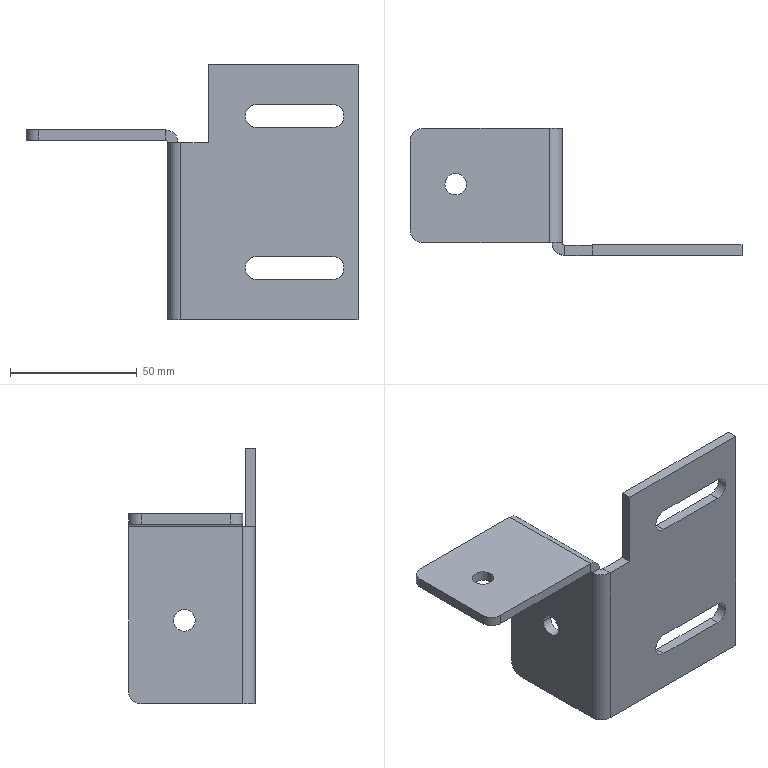Part | SolidWorks | features ICE 6, EdgeFlange 1, Fillet 1, FlatPattern 1, SMBaseFlange 1, SheetMetal 1 | 1 solid | 39 faces | box 131 x 50 x 101 mm | volume 48396 mm3 | plane 24 | cylinder 15 | commonest cylinder face diameters 10 x5 8.5 x4 9 x4 2 x2
STEP:
#1=CARTESIAN_POINT('',(-24.207,-4.491,33.));
#2=VERTEX_POINT('',#1);
#3=CARTESIAN_POINT('',(-24.207,4.009,33.));
#4=VERTEX_POINT('',#3);
#5=CARTESIAN_POINT('',(-24.207,-0.2414,33.));
#6=DIRECTION('',(1.,0.,0.));
#7=DIRECTION('',(0.,1.,0.));
#8=AXIS2_PLACEMENT_3D('',#5,#6,#7);
#9=CIRCLE('',#8,4.25);
#10=EDGE_CURVE('',#2,#4,#9,.T.);
#11=ORIENTED_EDGE('',*,*,#10,.F.);
#12=CARTESIAN_POINT('',(-20.207,-4.491,33.));
#13=VERTEX_POINT('',#12);
#14=CARTESIAN_POINT('',(-30.207,-4.491,33.));
#15=DIRECTION('',(1.,0.,0.));
#16=VECTOR('',#15,1000.);
#17=LINE('',#14,#16);
#18=EDGE_CURVE('',#2,#13,#17,.T.);
#19=ORIENTED_EDGE('',*,*,#18,.T.);
#20=CARTESIAN_POINT('',(-20.207,4.009,33.));
#21=VERTEX_POINT('',#20);
#22=CARTESIAN_POINT('',(-20.207,-0.2414,33.));
#23=DIRECTION('',(1.,0.,0.));
#24=DIRECTION('',(0.,1.,0.));
#25=AXIS2_PLACEMENT_3D('',#22,#23,#24);
#26=CIRCLE('',#25,4.25);
#27=EDGE_CURVE('',#13,#21,#26,.T.);
#28=ORIENTED_EDGE('',*,*,#27,.T.);
#29=CARTESIAN_POINT('',(-30.207,4.009,33.));
#30=DIRECTION('',(1.,0.,0.));
#31=VECTOR('',#30,1000.);
#32=LINE('',#29,#31);
#33=EDGE_CURVE('',#4,#21,#32,.T.);
#34=ORIENTED_EDGE('',*,*,#33,.F.);
#35=EDGE_LOOP('',(#11,#19,#28,#34));
#36=FACE_OUTER_BOUND('',#35,.T.);
#37=CARTESIAN_POINT('',(-30.207,-0.2414,33.));
#38=DIRECTION('',(1.,0.,0.));
#39=DIRECTION('',(0.,1.,0.));
#40=AXIS2_PLACEMENT_3D('',#37,#38,#39);
#41=CYLINDRICAL_SURFACE('',#40,4.25);
#42=ADVANCED_FACE('',(#36),#41,.F.);
#43=CARTESIAN_POINT('',(-66.457,-0.2414,71.));
#44=VERTEX_POINT('',#43);
#45=CARTESIAN_POINT('',(-57.957,-0.2414,71.));
#46=VERTEX_POINT('',#45);
#47=CARTESIAN_POINT('',(-62.207,-0.2414,71.));
#48=DIRECTION('',(0.,0.,1.));
#49=DIRECTION('',(1.,0.,0.));
#50=AXIS2_PLACEMENT_3D('',#47,#48,#49);
#51=CIRCLE('',#50,4.25);
#52=EDGE_CURVE('',#44,#46,#51,.T.);
#53=ORIENTED_EDGE('',*,*,#52,.F.);
#54=CARTESIAN_POINT('',(-66.457,-0.2414,75.));
#55=VERTEX_POINT('',#54);
#56=CARTESIAN_POINT('',(-66.457,-0.2414,65.));
#57=DIRECTION('',(0.,0.,1.));
#58=VECTOR('',#57,1000.);
#59=LINE('',#56,#58);
#60=EDGE_CURVE('',#44,#55,#59,.T.);
#61=ORIENTED_EDGE('',*,*,#60,.T.);
#62=CARTESIAN_POINT('',(-57.957,-0.2414,75.));
#63=VERTEX_POINT('',#62);
#64=CARTESIAN_POINT('',(-62.207,-0.2414,75.));
#65=DIRECTION('',(0.,0.,1.));
#66=DIRECTION('',(1.,0.,0.));
#67=AXIS2_PLACEMENT_3D('',#64,#65,#66);
#68=CIRCLE('',#67,4.25);
#69=EDGE_CURVE('',#55,#63,#68,.T.);
#70=ORIENTED_EDGE('',*,*,#69,.T.);
#71=CARTESIAN_POINT('',(-57.957,-0.2414,65.));
#72=DIRECTION('',(0.,0.,1.));
#73=VECTOR('',#72,1000.);
#74=LINE('',#71,#73);
#75=EDGE_CURVE('',#46,#63,#74,.T.);
#76=ORIENTED_EDGE('',*,*,#75,.F.);
#77=EDGE_LOOP('',(#53,#61,#70,#76));
#78=FACE_OUTER_BOUND('',#77,.T.);
#79=CARTESIAN_POINT('',(-62.207,-0.2414,65.));
#80=DIRECTION('',(0.,0.,1.));
#81=DIRECTION('',(1.,0.,0.));
#82=AXIS2_PLACEMENT_3D('',#79,#80,#81);
#83=CYLINDRICAL_SURFACE('',#82,4.25);
#84=ADVANCED_FACE('',(#78),#83,.F.);
#85=CARTESIAN_POINT('',(-8.207,-24.241,70.));
#86=VERTEX_POINT('',#85);
#87=CARTESIAN_POINT('',(-19.207,-24.241,70.));
#88=VERTEX_POINT('',#87);
#89=CARTESIAN_POINT('',(-24.207,-24.241,70.));
#90=DIRECTION('',(-1.,0.,0.));
#91=VECTOR('',#90,1000.);
#92=LINE('',#89,#91);
#93=EDGE_CURVE('',#86,#88,#92,.T.);
#94=ORIENTED_EDGE('',*,*,#93,.T.);
#95=CARTESIAN_POINT('',(-19.207,-28.241,70.));
#96=VERTEX_POINT('',#95);
#97=CARTESIAN_POINT('',(-19.207,-24.241,70.));
#98=DIRECTION('',(0.,-1.,0.));
#99=VECTOR('',#98,1000.);
#100=LINE('',#97,#99);
#101=EDGE_CURVE('',#88,#96,#100,.T.);
#102=ORIENTED_EDGE('',*,*,#101,.T.);
#103=CARTESIAN_POINT('',(-8.207,-28.241,70.));
#104=VERTEX_POINT('',#103);
#105=CARTESIAN_POINT('',(-8.207,-28.241,70.));
#106=DIRECTION('',(-1.,0.,0.));
#107=VECTOR('',#106,1000.);
#108=LINE('',#105,#107);
#109=EDGE_CURVE('',#104,#96,#108,.T.);
#110=ORIENTED_EDGE('',*,*,#109,.F.);
#111=CARTESIAN_POINT('',(-8.207,-28.241,70.));
#112=DIRECTION('',(0.,1.,0.));
#113=VECTOR('',#112,1000.);
#114=LINE('',#111,#113);
#115=EDGE_CURVE('',#104,#86,#114,.T.);
#116=ORIENTED_EDGE('',*,*,#115,.T.);
#117=EDGE_LOOP('',(#94,#102,#110,#116));
#118=FACE_OUTER_BOUND('',#117,.T.);
#119=CARTESIAN_POINT('',(-8.207,-28.241,70.));
#120=DIRECTION('',(0.,0.,-1.));
#121=DIRECTION('',(-1.,0.,0.));
#122=AXIS2_PLACEMENT_3D('',#119,#120,#121);
#123=PLANE('',#122);
#124=ADVANCED_FACE('',(#118),#123,.F.);
#125=CARTESIAN_POINT('',(-19.207,-28.241,0.));
#126=VERTEX_POINT('',#125);
#127=CARTESIAN_POINT('',(-19.207,-24.241,0.));
#128=VERTEX_POINT('',#127);
#129=CARTESIAN_POINT('',(-19.207,-28.241,0.));
#130=DIRECTION('',(0.,1.,0.));
#131=VECTOR('',#130,1000.);
#132=LINE('',#129,#131);
#133=EDGE_CURVE('',#126,#128,#132,.T.);
#134=ORIENTED_EDGE('',*,*,#133,.F.);
#135=CARTESIAN_POINT('',(-24.207,-23.241,0.));
#136=VERTEX_POINT('',#135);
#137=CARTESIAN_POINT('',(-19.207,-23.241,0.));
#138=DIRECTION('',(0.,0.,1.));
#139=DIRECTION('',(-1.,0.,0.));
#140=AXIS2_PLACEMENT_3D('',#137,#138,#139);
#141=CIRCLE('',#140,5.);
#142=EDGE_CURVE('',#136,#126,#141,.T.);
#143=ORIENTED_EDGE('',*,*,#142,.F.);
#144=CARTESIAN_POINT('',(-20.207,-23.241,0.));
#145=VERTEX_POINT('',#144);
#146=CARTESIAN_POINT('',(-20.207,-23.241,0.));
#147=DIRECTION('',(-1.,0.,0.));
#148=VECTOR('',#147,1000.);
#149=LINE('',#146,#148);
#150=EDGE_CURVE('',#145,#136,#149,.T.);
#151=ORIENTED_EDGE('',*,*,#150,.F.);
#152=CARTESIAN_POINT('',(-19.207,-23.241,0.));
#153=DIRECTION('',(0.,0.,1.));
#154=DIRECTION('',(1.,0.,0.));
#155=AXIS2_PLACEMENT_3D('',#152,#153,#154);
#156=CIRCLE('',#155,1.);
#157=EDGE_CURVE('',#145,#128,#156,.T.);
#158=ORIENTED_EDGE('',*,*,#157,.T.);
#159=EDGE_LOOP('',(#134,#143,#151,#158));
#160=FACE_OUTER_BOUND('',#159,.T.);
#161=CARTESIAN_POINT('',(-19.207,-28.241,0.));
#162=DIRECTION('',(0.,0.,-1.));
#163=DIRECTION('',(-1.,0.,0.));
#164=AXIS2_PLACEMENT_3D('',#161,#162,#163);
#165=PLANE('',#164);
#166=ADVANCED_FACE('',(#160),#165,.T.);
#167=CARTESIAN_POINT('',(50.793,-28.241,0.));
#168=VERTEX_POINT('',#167);
#169=CARTESIAN_POINT('',(50.793,-24.241,0.));
#170=VERTEX_POINT('',#169);
#171=CARTESIAN_POINT('',(50.793,-34.241,0.));
#172=DIRECTION('',(0.,1.,0.));
#173=VECTOR('',#172,1000.);
#174=LINE('',#171,#173);
#175=EDGE_CURVE('',#168,#170,#174,.T.);
#176=ORIENTED_EDGE('',*,*,#175,.F.);
#177=CARTESIAN_POINT('',(-24.207,-28.241,0.));
#178=DIRECTION('',(1.,0.,0.));
#179=VECTOR('',#178,1000.);
#180=LINE('',#177,#179);
#181=EDGE_CURVE('',#126,#168,#180,.T.);
#182=ORIENTED_EDGE('',*,*,#181,.F.);
#183=ORIENTED_EDGE('',*,*,#133,.T.);
#184=CARTESIAN_POINT('',(-24.207,-24.241,0.));
#185=DIRECTION('',(1.,0.,0.));
#186=VECTOR('',#185,1000.);
#187=LINE('',#184,#186);
#188=EDGE_CURVE('',#128,#170,#187,.T.);
#189=ORIENTED_EDGE('',*,*,#188,.T.);
#190=EDGE_LOOP('',(#176,#182,#183,#189));
#191=FACE_OUTER_BOUND('',#190,.T.);
#192=CARTESIAN_POINT('',(-20.207,-23.241,0.));
#193=DIRECTION('',(0.,0.,-1.));
#194=DIRECTION('',(-1.,0.,0.));
#195=AXIS2_PLACEMENT_3D('',#192,#193,#194);
#196=PLANE('',#195);
#197=ADVANCED_FACE('',(#191),#196,.T.);
#198=CARTESIAN_POINT('',(40.793,-28.241,16.));
#199=VERTEX_POINT('',#198);
#200=CARTESIAN_POINT('',(10.793,-28.241,16.));
#201=VERTEX_POINT('',#200);
#202=CARTESIAN_POINT('',(-24.207,-28.241,16.));
#203=DIRECTION('',(-1.,0.,0.));
#204=VECTOR('',#203,1000.);
#205=LINE('',#202,#204);
#206=EDGE_CURVE('',#199,#201,#205,.T.);
#207=ORIENTED_EDGE('',*,*,#206,.T.);
#208=CARTESIAN_POINT('',(10.793,-28.241,25.));
#209=VERTEX_POINT('',#208);
#210=CARTESIAN_POINT('',(10.793,-28.241,20.5));
#211=DIRECTION('',(0.,1.,0.));
#212=DIRECTION('',(0.,0.,1.));
#213=AXIS2_PLACEMENT_3D('',#210,#211,#212);
#214=CIRCLE('',#213,4.5);
#215=EDGE_CURVE('',#201,#209,#214,.T.);
#216=ORIENTED_EDGE('',*,*,#215,.T.);
#217=CARTESIAN_POINT('',(40.793,-28.241,25.));
#218=VERTEX_POINT('',#217);
#219=CARTESIAN_POINT('',(-24.207,-28.241,25.));
#220=DIRECTION('',(1.,0.,0.));
#221=VECTOR('',#220,1000.);
#222=LINE('',#219,#221);
#223=EDGE_CURVE('',#209,#218,#222,.T.);
#224=ORIENTED_EDGE('',*,*,#223,.T.);
#225=CARTESIAN_POINT('',(40.793,-28.241,20.5));
#226=DIRECTION('',(0.,1.,0.));
#227=DIRECTION('',(0.,0.,1.));
#228=AXIS2_PLACEMENT_3D('',#225,#226,#227);
#229=CIRCLE('',#228,4.5);
#230=EDGE_CURVE('',#218,#199,#229,.T.);
#231=ORIENTED_EDGE('',*,*,#230,.T.);
#232=EDGE_LOOP('',(#207,#216,#224,#231));
#233=FACE_BOUND('',#232,.T.);
#234=CARTESIAN_POINT('',(40.793,-28.241,76.));
#235=VERTEX_POINT('',#234);
#236=CARTESIAN_POINT('',(10.793,-28.241,76.));
#237=VERTEX_POINT('',#236);
#238=CARTESIAN_POINT('',(-24.207,-28.241,76.));
#239=DIRECTION('',(-1.,0.,0.));
#240=VECTOR('',#239,1000.);
#241=LINE('',#238,#240);
#242=EDGE_CURVE('',#235,#237,#241,.T.);
#243=ORIENTED_EDGE('',*,*,#242,.T.);
#244=CARTESIAN_POINT('',(10.793,-28.241,85.));
#245=VERTEX_POINT('',#244);
#246=CARTESIAN_POINT('',(10.793,-28.241,80.5));
#247=DIRECTION('',(0.,1.,0.));
#248=DIRECTION('',(0.,0.,1.));
#249=AXIS2_PLACEMENT_3D('',#246,#247,#248);
#250=CIRCLE('',#249,4.5);
#251=EDGE_CURVE('',#237,#245,#250,.T.);
#252=ORIENTED_EDGE('',*,*,#251,.T.);
#253=CARTESIAN_POINT('',(40.793,-28.241,85.));
#254=VERTEX_POINT('',#253);
#255=CARTESIAN_POINT('',(-24.207,-28.241,85.));
#256=DIRECTION('',(1.,0.,0.));
#257=VECTOR('',#256,1000.);
#258=LINE('',#255,#257);
#259=EDGE_CURVE('',#245,#254,#258,.T.);
#260=ORIENTED_EDGE('',*,*,#259,.T.);
#261=CARTESIAN_POINT('',(40.793,-28.241,80.5));
#262=DIRECTION('',(0.,1.,0.));
#263=DIRECTION('',(0.,0.,1.));
#264=AXIS2_PLACEMENT_3D('',#261,#262,#263);
#265=CIRCLE('',#264,4.5);
#266=EDGE_CURVE('',#254,#235,#265,.T.);
#267=ORIENTED_EDGE('',*,*,#266,.T.);
#268=EDGE_LOOP('',(#243,#252,#260,#267));
#269=FACE_BOUND('',#268,.T.);
#270=ORIENTED_EDGE('',*,*,#181,.T.);
#271=CARTESIAN_POINT('',(50.793,-28.241,101.));
#272=VERTEX_POINT('',#271);
#273=CARTESIAN_POINT('',(50.793,-28.241,125.));
#274=DIRECTION('',(0.,0.,1.));
#275=VECTOR('',#274,1000.);
#276=LINE('',#273,#275);
#277=EDGE_CURVE('',#168,#272,#276,.T.);
#278=ORIENTED_EDGE('',*,*,#277,.T.);
#279=CARTESIAN_POINT('',(-8.207,-28.241,101.));
#280=VERTEX_POINT('',#279);
#281=CARTESIAN_POINT('',(-24.207,-28.241,101.));
#282=DIRECTION('',(-1.,0.,0.));
#283=VECTOR('',#282,1000.);
#284=LINE('',#281,#283);
#285=EDGE_CURVE('',#272,#280,#284,.T.);
#286=ORIENTED_EDGE('',*,*,#285,.T.);
#287=CARTESIAN_POINT('',(-8.207,-28.241,125.));
#288=DIRECTION('',(0.,0.,-1.));
#289=VECTOR('',#288,1000.);
#290=LINE('',#287,#289);
#291=EDGE_CURVE('',#280,#104,#290,.T.);
#292=ORIENTED_EDGE('',*,*,#291,.T.);
#293=ORIENTED_EDGE('',*,*,#109,.T.);
#294=CARTESIAN_POINT('',(-19.207,-28.241,125.));
#295=DIRECTION('',(0.,0.,-1.));
#296=VECTOR('',#295,1000.);
#297=LINE('',#294,#296);
#298=EDGE_CURVE('',#96,#126,#297,.T.);
#299=ORIENTED_EDGE('',*,*,#298,.T.);
#300=EDGE_LOOP('',(#270,#278,#286,#292,#293,#299));
#301=FACE_OUTER_BOUND('',#300,.T.);
#302=CARTESIAN_POINT('',(-24.207,-28.241,125.));
#303=DIRECTION('',(0.,1.,0.));
#304=DIRECTION('',(0.,0.,1.));
#305=AXIS2_PLACEMENT_3D('',#302,#303,#304);
#306=PLANE('',#305);
#307=ADVANCED_FACE('',(#233,#269,#301),#306,.F.);
#308=CARTESIAN_POINT('',(10.793,-24.241,16.));
#309=VERTEX_POINT('',#308);
#310=CARTESIAN_POINT('',(10.793,-24.241,25.));
#311=VERTEX_POINT('',#310);
#312=CARTESIAN_POINT('',(10.793,-24.241,20.5));
#313=DIRECTION('',(0.,1.,0.));
#314=DIRECTION('',(0.,0.,1.));
#315=AXIS2_PLACEMENT_3D('',#312,#313,#314);
#316=CIRCLE('',#315,4.5);
#317=EDGE_CURVE('',#309,#311,#316,.T.);
#318=ORIENTED_EDGE('',*,*,#317,.F.);
#319=CARTESIAN_POINT('',(40.793,-24.241,16.));
#320=VERTEX_POINT('',#319);
#321=CARTESIAN_POINT('',(10.793,-24.241,16.));
#322=DIRECTION('',(-1.,0.,0.));
#323=VECTOR('',#322,1000.);
#324=LINE('',#321,#323);
#325=EDGE_CURVE('',#320,#309,#324,.T.);
#326=ORIENTED_EDGE('',*,*,#325,.F.);
#327=CARTESIAN_POINT('',(40.793,-24.241,25.));
#328=VERTEX_POINT('',#327);
#329=CARTESIAN_POINT('',(40.793,-24.241,20.5));
#330=DIRECTION('',(0.,1.,0.));
#331=DIRECTION('',(0.,0.,1.));
#332=AXIS2_PLACEMENT_3D('',#329,#330,#331);
#333=CIRCLE('',#332,4.5);
#334=EDGE_CURVE('',#328,#320,#333,.T.);
#335=ORIENTED_EDGE('',*,*,#334,.F.);
#336=CARTESIAN_POINT('',(10.793,-24.241,25.));
#337=DIRECTION('',(1.,0.,0.));
#338=VECTOR('',#337,1000.);
#339=LINE('',#336,#338);
#340=EDGE_CURVE('',#311,#328,#339,.T.);
#341=ORIENTED_EDGE('',*,*,#340,.F.);
#342=EDGE_LOOP('',(#318,#326,#335,#341));
#343=FACE_BOUND('',#342,.T.);
#344=CARTESIAN_POINT('',(10.793,-24.241,76.));
#345=VERTEX_POINT('',#344);
#346=CARTESIAN_POINT('',(10.793,-24.241,85.));
#347=VERTEX_POINT('',#346);
#348=CARTESIAN_POINT('',(10.793,-24.241,80.5));
#349=DIRECTION('',(0.,1.,0.));
#350=DIRECTION('',(0.,0.,-1.));
#351=AXIS2_PLACEMENT_3D('',#348,#349,#350);
#352=CIRCLE('',#351,4.5);
#353=EDGE_CURVE('',#345,#347,#352,.T.);
#354=ORIENTED_EDGE('',*,*,#353,.F.);
#355=CARTESIAN_POINT('',(40.793,-24.241,76.));
#356=VERTEX_POINT('',#355);
#357=CARTESIAN_POINT('',(10.793,-24.241,76.));
#358=DIRECTION('',(-1.,0.,0.));
#359=VECTOR('',#358,1000.);
#360=LINE('',#357,#359);
#361=EDGE_CURVE('',#356,#345,#360,.T.);
#362=ORIENTED_EDGE('',*,*,#361,.F.);
#363=CARTESIAN_POINT('',(40.793,-24.241,85.));
#364=VERTEX_POINT('',#363);
#365=CARTESIAN_POINT('',(40.793,-24.241,80.5));
#366=DIRECTION('',(0.,1.,0.));
#367=DIRECTION('',(0.,0.,-1.));
#368=AXIS2_PLACEMENT_3D('',#365,#366,#367);
#369=CIRCLE('',#368,4.5);
#370=EDGE_CURVE('',#364,#356,#369,.T.);
#371=ORIENTED_EDGE('',*,*,#370,.F.);
#372=CARTESIAN_POINT('',(10.793,-24.241,85.));
#373=DIRECTION('',(1.,0.,0.));
#374=VECTOR('',#373,1000.);
#375=LINE('',#372,#374);
#376=EDGE_CURVE('',#347,#364,#375,.T.);
#377=ORIENTED_EDGE('',*,*,#376,.F.);
#378=EDGE_LOOP('',(#354,#362,#371,#377));
#379=FACE_BOUND('',#378,.T.);
#380=CARTESIAN_POINT('',(50.793,-24.241,101.));
#381=VERTEX_POINT('',#380);
#382=CARTESIAN_POINT('',(50.793,-24.241,0.));
#383=DIRECTION('',(0.,0.,1.));
#384=VECTOR('',#383,1000.);
#385=LINE('',#382,#384);
#386=EDGE_CURVE('',#170,#381,#385,.T.);
#387=ORIENTED_EDGE('',*,*,#386,.F.);
#388=ORIENTED_EDGE('',*,*,#188,.F.);
#389=CARTESIAN_POINT('',(-19.207,-24.241,125.));
#390=DIRECTION('',(0.,0.,-1.));
#391=VECTOR('',#390,1000.);
#392=LINE('',#389,#391);
#393=EDGE_CURVE('',#88,#128,#392,.T.);
#394=ORIENTED_EDGE('',*,*,#393,.F.);
#395=ORIENTED_EDGE('',*,*,#93,.F.);
#396=CARTESIAN_POINT('',(-8.207,-24.241,101.));
#397=VERTEX_POINT('',#396);
#398=CARTESIAN_POINT('',(-8.207,-24.241,125.));
#399=DIRECTION('',(0.,0.,-1.));
#400=VECTOR('',#399,1000.);
#401=LINE('',#398,#400);
#402=EDGE_CURVE('',#397,#86,#401,.T.);
#403=ORIENTED_EDGE('',*,*,#402,.F.);
#404=CARTESIAN_POINT('',(-8.207,-24.241,101.));
#405=DIRECTION('',(-1.,0.,0.));
#406=VECTOR('',#405,1000.);
#407=LINE('',#404,#406);
#408=EDGE_CURVE('',#381,#397,#407,.T.);
#409=ORIENTED_EDGE('',*,*,#408,.F.);
#410=EDGE_LOOP('',(#387,#388,#394,#395,#403,#409));
#411=FACE_OUTER_BOUND('',#410,.T.);
#412=CARTESIAN_POINT('',(-24.207,-24.241,125.));
#413=DIRECTION('',(0.,1.,0.));
#414=DIRECTION('',(0.,0.,1.));
#415=AXIS2_PLACEMENT_3D('',#412,#413,#414);
#416=PLANE('',#415);
#417=ADVANCED_FACE('',(#343,#379,#411),#416,.T.);
#418=CARTESIAN_POINT('',(-20.207,-23.241,70.));
#419=VERTEX_POINT('',#418);
#420=CARTESIAN_POINT('',(-19.207,-23.241,70.));
#421=DIRECTION('',(0.,0.,-1.));
#422=DIRECTION('',(-1.,0.,0.));
#423=AXIS2_PLACEMENT_3D('',#420,#421,#422);
#424=CIRCLE('',#423,1.);
#425=EDGE_CURVE('',#88,#419,#424,.T.);
#426=ORIENTED_EDGE('',*,*,#425,.F.);
#427=ORIENTED_EDGE('',*,*,#393,.T.);
#428=ORIENTED_EDGE('',*,*,#157,.F.);
#429=CARTESIAN_POINT('',(-20.207,-23.241,125.));
#430=DIRECTION('',(0.,0.,-1.));
#431=VECTOR('',#430,1000.);
#432=LINE('',#429,#431);
#433=EDGE_CURVE('',#419,#145,#432,.T.);
#434=ORIENTED_EDGE('',*,*,#433,.F.);
#435=EDGE_LOOP('',(#426,#427,#428,#434));
#436=FACE_OUTER_BOUND('',#435,.T.);
#437=CARTESIAN_POINT('',(-19.207,-23.241,125.));
#438=DIRECTION('',(0.,0.,-1.));
#439=DIRECTION('',(-1.,0.,0.));
#440=AXIS2_PLACEMENT_3D('',#437,#438,#439);
#441=CYLINDRICAL_SURFACE('',#440,1.);
#442=ADVANCED_FACE('',(#436),#441,.F.);
#443=CARTESIAN_POINT('',(-20.207,-0.2414,33.));
#444=DIRECTION('',(1.,0.,0.));
#445=DIRECTION('',(0.,1.,0.));
#446=AXIS2_PLACEMENT_3D('',#443,#444,#445);
#447=CIRCLE('',#446,4.25);
#448=EDGE_CURVE('',#21,#13,#447,.T.);
#449=ORIENTED_EDGE('',*,*,#448,.F.);
#450=ORIENTED_EDGE('',*,*,#27,.F.);
#451=EDGE_LOOP('',(#449,#450));
#452=FACE_BOUND('',#451,.T.);
#453=CARTESIAN_POINT('',(-20.207,16.759,0.));
#454=VERTEX_POINT('',#453);
#455=CARTESIAN_POINT('',(-20.207,21.759,0.));
#456=DIRECTION('',(0.,-1.,0.));
#457=VECTOR('',#456,1000.);
#458=LINE('',#455,#457);
#459=EDGE_CURVE('',#454,#145,#458,.T.);
#460=ORIENTED_EDGE('',*,*,#459,.F.);
#461=CARTESIAN_POINT('',(-20.207,21.759,5.));
#462=VERTEX_POINT('',#461);
#463=CARTESIAN_POINT('',(-20.207,16.759,5.));
#464=DIRECTION('',(1.,0.,0.));
#465=DIRECTION('',(0.,1.,0.));
#466=AXIS2_PLACEMENT_3D('',#463,#464,#465);
#467=CIRCLE('',#466,5.);
#468=EDGE_CURVE('',#454,#462,#467,.T.);
#469=ORIENTED_EDGE('',*,*,#468,.T.);
#470=CARTESIAN_POINT('',(-20.207,21.759,70.));
#471=VERTEX_POINT('',#470);
#472=CARTESIAN_POINT('',(-20.207,21.759,125.));
#473=DIRECTION('',(0.,0.,-1.));
#474=VECTOR('',#473,1000.);
#475=LINE('',#472,#474);
#476=EDGE_CURVE('',#471,#462,#475,.T.);
#477=ORIENTED_EDGE('',*,*,#476,.F.);
#478=CARTESIAN_POINT('',(-20.207,21.759,70.));
#479=DIRECTION('',(0.,1.,0.));
#480=VECTOR('',#479,1000.);
#481=LINE('',#478,#480);
#482=EDGE_CURVE('',#419,#471,#481,.T.);
#483=ORIENTED_EDGE('',*,*,#482,.F.);
#484=ORIENTED_EDGE('',*,*,#433,.T.);
#485=EDGE_LOOP('',(#460,#469,#477,#483,#484));
#486=FACE_OUTER_BOUND('',#485,.T.);
#487=CARTESIAN_POINT('',(-20.207,21.759,125.));
#488=DIRECTION('',(1.,0.,0.));
#489=DIRECTION('',(0.,1.,0.));
#490=AXIS2_PLACEMENT_3D('',#487,#488,#489);
#491=PLANE('',#490);
#492=ADVANCED_FACE('',(#452,#486),#491,.T.);
#493=ORIENTED_EDGE('',*,*,#476,.T.);
#494=CARTESIAN_POINT('',(-24.207,21.759,5.));
#495=VERTEX_POINT('',#494);
#496=CARTESIAN_POINT('',(-24.207,21.759,5.));
#497=DIRECTION('',(-1.,0.,0.));
#498=VECTOR('',#497,1000.);
#499=LINE('',#496,#498);
#500=EDGE_CURVE('',#462,#495,#499,.T.);
#501=ORIENTED_EDGE('',*,*,#500,.T.);
#502=CARTESIAN_POINT('',(-24.207,21.759,70.));
#503=VERTEX_POINT('',#502);
#504=CARTESIAN_POINT('',(-24.207,21.759,125.));
#505=DIRECTION('',(0.,0.,-1.));
#506=VECTOR('',#505,1000.);
#507=LINE('',#504,#506);
#508=EDGE_CURVE('',#503,#495,#507,.T.);
#509=ORIENTED_EDGE('',*,*,#508,.F.);
#510=CARTESIAN_POINT('',(-8.207,21.759,70.));
#511=DIRECTION('',(-1.,0.,0.));
#512=VECTOR('',#511,1000.);
#513=LINE('',#510,#512);
#514=EDGE_CURVE('',#471,#503,#513,.T.);
#515=ORIENTED_EDGE('',*,*,#514,.F.);
#516=EDGE_LOOP('',(#493,#501,#509,#515));
#517=FACE_OUTER_BOUND('',#516,.T.);
#518=CARTESIAN_POINT('',(-24.207,21.759,125.));
#519=DIRECTION('',(0.,1.,0.));
#520=DIRECTION('',(0.,0.,1.));
#521=AXIS2_PLACEMENT_3D('',#518,#519,#520);
#522=PLANE('',#521);
#523=ADVANCED_FACE('',(#517),#522,.T.);
#524=CARTESIAN_POINT('',(-24.207,-0.2414,33.));
#525=DIRECTION('',(1.,0.,0.));
#526=DIRECTION('',(0.,1.,0.));
#527=AXIS2_PLACEMENT_3D('',#524,#525,#526);
#528=CIRCLE('',#527,4.25);
#529=EDGE_CURVE('',#4,#2,#528,.T.);
#530=ORIENTED_EDGE('',*,*,#529,.T.);
#531=ORIENTED_EDGE('',*,*,#10,.T.);
#532=EDGE_LOOP('',(#530,#531));
#533=FACE_BOUND('',#532,.T.);
#534=ORIENTED_EDGE('',*,*,#508,.T.);
#535=CARTESIAN_POINT('',(-24.207,16.759,0.));
#536=VERTEX_POINT('',#535);
#537=CARTESIAN_POINT('',(-24.207,16.759,5.));
#538=DIRECTION('',(-1.,0.,0.));
#539=DIRECTION('',(0.,1.,0.));
#540=AXIS2_PLACEMENT_3D('',#537,#538,#539);
#541=CIRCLE('',#540,5.);
#542=EDGE_CURVE('',#495,#536,#541,.T.);
#543=ORIENTED_EDGE('',*,*,#542,.T.);
#544=CARTESIAN_POINT('',(-24.207,21.759,0.));
#545=DIRECTION('',(0.,-1.,0.));
#546=VECTOR('',#545,1000.);
#547=LINE('',#544,#546);
#548=EDGE_CURVE('',#536,#136,#547,.T.);
#549=ORIENTED_EDGE('',*,*,#548,.T.);
#550=CARTESIAN_POINT('',(-24.207,-23.241,70.));
#551=VERTEX_POINT('',#550);
#552=CARTESIAN_POINT('',(-24.207,-23.241,125.));
#553=DIRECTION('',(0.,0.,-1.));
#554=VECTOR('',#553,1000.);
#555=LINE('',#552,#554);
#556=EDGE_CURVE('',#551,#136,#555,.T.);
#557=ORIENTED_EDGE('',*,*,#556,.F.);
#558=CARTESIAN_POINT('',(-24.207,21.759,70.));
#559=DIRECTION('',(0.,1.,0.));
#560=VECTOR('',#559,1000.);
#561=LINE('',#558,#560);
#562=EDGE_CURVE('',#551,#503,#561,.T.);
#563=ORIENTED_EDGE('',*,*,#562,.T.);
#564=EDGE_LOOP('',(#534,#543,#549,#557,#563));
#565=FACE_OUTER_BOUND('',#564,.T.);
#566=CARTESIAN_POINT('',(-24.207,21.759,125.));
#567=DIRECTION('',(1.,0.,0.));
#568=DIRECTION('',(0.,1.,0.));
#569=AXIS2_PLACEMENT_3D('',#566,#567,#568);
#570=PLANE('',#569);
#571=ADVANCED_FACE('',(#533,#565),#570,.F.);
#572=ORIENTED_EDGE('',*,*,#298,.F.);
#573=CARTESIAN_POINT('',(-19.207,-23.241,70.));
#574=DIRECTION('',(0.,0.,-1.));
#575=DIRECTION('',(-1.,0.,0.));
#576=AXIS2_PLACEMENT_3D('',#573,#574,#575);
#577=CIRCLE('',#576,5.);
#578=EDGE_CURVE('',#96,#551,#577,.T.);
#579=ORIENTED_EDGE('',*,*,#578,.T.);
#580=ORIENTED_EDGE('',*,*,#556,.T.);
#581=ORIENTED_EDGE('',*,*,#142,.T.);
#582=EDGE_LOOP('',(#572,#579,#580,#581));
#583=FACE_OUTER_BOUND('',#582,.T.);
#584=CARTESIAN_POINT('',(-19.207,-23.241,125.));
#585=DIRECTION('',(0.,0.,-1.));
#586=DIRECTION('',(-1.,0.,0.));
#587=AXIS2_PLACEMENT_3D('',#584,#585,#586);
#588=CYLINDRICAL_SURFACE('',#587,5.);
#589=ADVANCED_FACE('',(#583),#588,.T.);
#590=ORIENTED_EDGE('',*,*,#548,.F.);
#591=CARTESIAN_POINT('',(-20.207,16.759,0.));
#592=DIRECTION('',(1.,0.,0.));
#593=VECTOR('',#592,1000.);
#594=LINE('',#591,#593);
#595=EDGE_CURVE('',#536,#454,#594,.T.);
#596=ORIENTED_EDGE('',*,*,#595,.T.);
#597=ORIENTED_EDGE('',*,*,#459,.T.);
#598=ORIENTED_EDGE('',*,*,#150,.T.);
#599=EDGE_LOOP('',(#590,#596,#597,#598));
#600=FACE_OUTER_BOUND('',#599,.T.);
#601=CARTESIAN_POINT('',(-19.207,-23.241,0.));
#602=DIRECTION('',(0.,0.,1.));
#603=DIRECTION('',(1.,0.,0.));
#604=AXIS2_PLACEMENT_3D('',#601,#602,#603);
#605=PLANE('',#604);
#606=ADVANCED_FACE('',(#600),#605,.F.);
#607=CARTESIAN_POINT('',(-24.207,-23.241,70.));
#608=DIRECTION('',(1.,0.,0.));
#609=VECTOR('',#608,1000.);
#610=LINE('',#607,#609);
#611=EDGE_CURVE('',#551,#419,#610,.T.);
#612=ORIENTED_EDGE('',*,*,#611,.F.);
#613=ORIENTED_EDGE('',*,*,#578,.F.);
#614=ORIENTED_EDGE('',*,*,#101,.F.);
#615=ORIENTED_EDGE('',*,*,#425,.T.);
#616=EDGE_LOOP('',(#612,#613,#614,#615));
#617=FACE_OUTER_BOUND('',#616,.T.);
#618=CARTESIAN_POINT('',(-8.207,-28.241,70.));
#619=DIRECTION('',(0.,0.,-1.));
#620=DIRECTION('',(-1.,0.,0.));
#621=AXIS2_PLACEMENT_3D('',#618,#619,#620);
#622=PLANE('',#621);
#623=ADVANCED_FACE('',(#617),#622,.F.);
#624=ORIENTED_EDGE('',*,*,#291,.F.);
#625=CARTESIAN_POINT('',(-8.207,-28.241,101.));
#626=DIRECTION('',(0.,1.,0.));
#627=VECTOR('',#626,1000.);
#628=LINE('',#625,#627);
#629=EDGE_CURVE('',#280,#397,#628,.T.);
#630=ORIENTED_EDGE('',*,*,#629,.T.);
#631=ORIENTED_EDGE('',*,*,#402,.T.);
#632=ORIENTED_EDGE('',*,*,#115,.F.);
#633=EDGE_LOOP('',(#624,#630,#631,#632));
#634=FACE_OUTER_BOUND('',#633,.T.);
#635=CARTESIAN_POINT('',(-8.207,-28.241,125.));
#636=DIRECTION('',(1.,0.,0.));
#637=DIRECTION('',(0.,0.,-1.));
#638=AXIS2_PLACEMENT_3D('',#635,#636,#637);
#639=PLANE('',#638);
#640=ADVANCED_FACE('',(#634),#639,.F.);
#641=CARTESIAN_POINT('',(-25.207,-23.241,71.));
#642=VERTEX_POINT('',#641);
#643=CARTESIAN_POINT('',(-25.207,-23.241,75.));
#644=VERTEX_POINT('',#643);
#645=CARTESIAN_POINT('',(-25.207,-23.241,75.));
#646=DIRECTION('',(0.,0.,1.));
#647=VECTOR('',#646,1000.);
#648=LINE('',#645,#647);
#649=EDGE_CURVE('',#642,#644,#648,.T.);
#650=ORIENTED_EDGE('',*,*,#649,.F.);
#651=CARTESIAN_POINT('',(-25.207,-23.241,70.));
#652=DIRECTION('',(0.,-1.,0.));
#653=DIRECTION('',(0.,0.,1.));
#654=AXIS2_PLACEMENT_3D('',#651,#652,#653);
#655=CIRCLE('',#654,1.);
#656=EDGE_CURVE('',#551,#642,#655,.T.);
#657=ORIENTED_EDGE('',*,*,#656,.F.);
#658=ORIENTED_EDGE('',*,*,#611,.T.);
#659=CARTESIAN_POINT('',(-25.207,-23.241,70.));
#660=DIRECTION('',(0.,-1.,0.));
#661=DIRECTION('',(0.,0.,1.));
#662=AXIS2_PLACEMENT_3D('',#659,#660,#661);
#663=CIRCLE('',#662,5.);
#664=EDGE_CURVE('',#419,#644,#663,.T.);
#665=ORIENTED_EDGE('',*,*,#664,.T.);
#666=EDGE_LOOP('',(#650,#657,#658,#665));
#667=FACE_OUTER_BOUND('',#666,.T.);
#668=CARTESIAN_POINT('',(-25.207,-23.241,70.));
#669=DIRECTION('',(0.,-1.,0.));
#670=DIRECTION('',(0.,0.,-1.));
#671=AXIS2_PLACEMENT_3D('',#668,#669,#670);
#672=PLANE('',#671);
#673=ADVANCED_FACE('',(#667),#672,.T.);
#674=CARTESIAN_POINT('',(-25.207,21.759,71.));
#675=VERTEX_POINT('',#674);
#676=CARTESIAN_POINT('',(-25.207,21.759,70.));
#677=DIRECTION('',(0.,1.,0.));
#678=DIRECTION('',(0.,0.,1.));
#679=AXIS2_PLACEMENT_3D('',#676,#677,#678);
#680=CIRCLE('',#679,1.);
#681=EDGE_CURVE('',#675,#503,#680,.T.);
#682=ORIENTED_EDGE('',*,*,#681,.F.);
#683=CARTESIAN_POINT('',(-25.207,21.759,75.));
#684=VERTEX_POINT('',#683);
#685=CARTESIAN_POINT('',(-25.207,21.759,71.));
#686=DIRECTION('',(0.,0.,1.));
#687=VECTOR('',#686,1000.);
#688=LINE('',#685,#687);
#689=EDGE_CURVE('',#675,#684,#688,.T.);
#690=ORIENTED_EDGE('',*,*,#689,.T.);
#691=CARTESIAN_POINT('',(-25.207,21.759,70.));
#692=DIRECTION('',(0.,1.,0.));
#693=DIRECTION('',(0.,0.,1.));
#694=AXIS2_PLACEMENT_3D('',#691,#692,#693);
#695=CIRCLE('',#694,5.);
#696=EDGE_CURVE('',#684,#471,#695,.T.);
#697=ORIENTED_EDGE('',*,*,#696,.T.);
#698=ORIENTED_EDGE('',*,*,#514,.T.);
#699=EDGE_LOOP('',(#682,#690,#697,#698));
#700=FACE_OUTER_BOUND('',#699,.T.);
#701=CARTESIAN_POINT('',(-25.207,21.759,70.));
#702=DIRECTION('',(0.,-1.,0.));
#703=DIRECTION('',(0.,0.,-1.));
#704=AXIS2_PLACEMENT_3D('',#701,#702,#703);
#705=PLANE('',#704);
#706=ADVANCED_FACE('',(#700),#705,.F.);
#707=ORIENTED_EDGE('',*,*,#482,.T.);
#708=ORIENTED_EDGE('',*,*,#696,.F.);
#709=CARTESIAN_POINT('',(-25.207,0.,75.));
#710=DIRECTION('',(0.,1.,0.));
#711=VECTOR('',#710,1000.);
#712=LINE('',#709,#711);
#713=EDGE_CURVE('',#644,#684,#712,.T.);
#714=ORIENTED_EDGE('',*,*,#713,.F.);
#715=ORIENTED_EDGE('',*,*,#664,.F.);
#716=EDGE_LOOP('',(#707,#708,#714,#715));
#717=FACE_OUTER_BOUND('',#716,.T.);
#718=CARTESIAN_POINT('',(-25.207,21.759,70.));
#719=DIRECTION('',(0.,1.,0.));
#720=DIRECTION('',(0.,0.,1.));
#721=AXIS2_PLACEMENT_3D('',#718,#719,#720);
#722=CYLINDRICAL_SURFACE('',#721,5.);
#723=ADVANCED_FACE('',(#717),#722,.T.);
#724=ORIENTED_EDGE('',*,*,#562,.F.);
#725=ORIENTED_EDGE('',*,*,#656,.T.);
#726=CARTESIAN_POINT('',(-25.207,-23.241,71.));
#727=DIRECTION('',(0.,1.,0.));
#728=VECTOR('',#727,1000.);
#729=LINE('',#726,#728);
#730=EDGE_CURVE('',#642,#675,#729,.T.);
#731=ORIENTED_EDGE('',*,*,#730,.T.);
#732=ORIENTED_EDGE('',*,*,#681,.T.);
#733=EDGE_LOOP('',(#724,#725,#731,#732));
#734=FACE_OUTER_BOUND('',#733,.T.);
#735=CARTESIAN_POINT('',(-25.207,21.759,70.));
#736=DIRECTION('',(0.,1.,0.));
#737=DIRECTION('',(0.,0.,1.));
#738=AXIS2_PLACEMENT_3D('',#735,#736,#737);
#739=CYLINDRICAL_SURFACE('',#738,1.);
#740=ADVANCED_FACE('',(#734),#739,.F.);
#741=CARTESIAN_POINT('',(-75.207,21.759,71.));
#742=VERTEX_POINT('',#741);
#743=CARTESIAN_POINT('',(0.,21.759,71.));
#744=DIRECTION('',(1.,0.,0.));
#745=VECTOR('',#744,1000.);
#746=LINE('',#743,#745);
#747=EDGE_CURVE('',#742,#675,#746,.T.);
#748=ORIENTED_EDGE('',*,*,#747,.F.);
#749=CARTESIAN_POINT('',(-75.207,21.759,75.));
#750=VERTEX_POINT('',#749);
#751=CARTESIAN_POINT('',(-75.207,21.759,75.));
#752=DIRECTION('',(0.,0.,1.));
#753=VECTOR('',#752,1000.);
#754=LINE('',#751,#753);
#755=EDGE_CURVE('',#742,#750,#754,.T.);
#756=ORIENTED_EDGE('',*,*,#755,.T.);
#757=CARTESIAN_POINT('',(-24.207,21.759,75.));
#758=DIRECTION('',(1.,0.,0.));
#759=VECTOR('',#758,1000.);
#760=LINE('',#757,#759);
#761=EDGE_CURVE('',#750,#684,#760,.T.);
#762=ORIENTED_EDGE('',*,*,#761,.T.);
#763=ORIENTED_EDGE('',*,*,#689,.F.);
#764=EDGE_LOOP('',(#748,#756,#762,#763));
#765=FACE_OUTER_BOUND('',#764,.T.);
#766=CARTESIAN_POINT('',(-24.207,21.759,75.));
#767=DIRECTION('',(0.,1.,0.));
#768=DIRECTION('',(-1.,0.,0.));
#769=AXIS2_PLACEMENT_3D('',#766,#767,#768);
#770=PLANE('',#769);
#771=ADVANCED_FACE('',(#765),#770,.T.);
#772=CARTESIAN_POINT('',(-75.207,-23.241,75.));
#773=VERTEX_POINT('',#772);
#774=CARTESIAN_POINT('',(-80.207,-23.241,75.));
#775=DIRECTION('',(-1.,0.,0.));
#776=VECTOR('',#775,1000.);
#777=LINE('',#774,#776);
#778=EDGE_CURVE('',#644,#773,#777,.T.);
#779=ORIENTED_EDGE('',*,*,#778,.T.);
#780=CARTESIAN_POINT('',(-75.207,-23.241,71.));
#781=VERTEX_POINT('',#780);
#782=CARTESIAN_POINT('',(-75.207,-23.241,75.));
#783=DIRECTION('',(0.,0.,-1.));
#784=VECTOR('',#783,1000.);
#785=LINE('',#782,#784);
#786=EDGE_CURVE('',#773,#781,#785,.T.);
#787=ORIENTED_EDGE('',*,*,#786,.T.);
#788=CARTESIAN_POINT('',(0.,-23.241,71.));
#789=DIRECTION('',(-1.,0.,0.));
#790=VECTOR('',#789,1000.);
#791=LINE('',#788,#790);
#792=EDGE_CURVE('',#642,#781,#791,.T.);
#793=ORIENTED_EDGE('',*,*,#792,.F.);
#794=ORIENTED_EDGE('',*,*,#649,.T.);
#795=EDGE_LOOP('',(#779,#787,#793,#794));
#796=FACE_OUTER_BOUND('',#795,.T.);
#797=CARTESIAN_POINT('',(-80.207,-23.241,75.));
#798=DIRECTION('',(0.,-1.,0.));
#799=DIRECTION('',(1.,0.,0.));
#800=AXIS2_PLACEMENT_3D('',#797,#798,#799);
#801=PLANE('',#800);
#802=ADVANCED_FACE('',(#796),#801,.T.);
#803=CARTESIAN_POINT('',(-62.207,-0.2414,75.));
#804=DIRECTION('',(0.,0.,1.));
#805=DIRECTION('',(1.,0.,0.));
#806=AXIS2_PLACEMENT_3D('',#803,#804,#805);
#807=CIRCLE('',#806,4.25);
#808=EDGE_CURVE('',#63,#55,#807,.T.);
#809=ORIENTED_EDGE('',*,*,#808,.F.);
#810=ORIENTED_EDGE('',*,*,#69,.F.);
#811=EDGE_LOOP('',(#809,#810));
#812=FACE_BOUND('',#811,.T.);
#813=CARTESIAN_POINT('',(-80.207,-18.241,75.));
#814=VERTEX_POINT('',#813);
#815=CARTESIAN_POINT('',(-80.207,16.759,75.));
#816=VERTEX_POINT('',#815);
#817=CARTESIAN_POINT('',(-80.207,21.759,75.));
#818=DIRECTION('',(0.,1.,0.));
#819=VECTOR('',#818,1000.);
#820=LINE('',#817,#819);
#821=EDGE_CURVE('',#814,#816,#820,.T.);
#822=ORIENTED_EDGE('',*,*,#821,.F.);
#823=CARTESIAN_POINT('',(-75.207,-18.241,75.));
#824=DIRECTION('',(0.,0.,1.));
#825=DIRECTION('',(1.,0.,0.));
#826=AXIS2_PLACEMENT_3D('',#823,#824,#825);
#827=CIRCLE('',#826,5.);
#828=EDGE_CURVE('',#814,#773,#827,.T.);
#829=ORIENTED_EDGE('',*,*,#828,.T.);
#830=ORIENTED_EDGE('',*,*,#778,.F.);
#831=ORIENTED_EDGE('',*,*,#713,.T.);
#832=ORIENTED_EDGE('',*,*,#761,.F.);
#833=CARTESIAN_POINT('',(-75.207,16.759,75.));
#834=DIRECTION('',(0.,0.,1.));
#835=DIRECTION('',(1.,0.,0.));
#836=AXIS2_PLACEMENT_3D('',#833,#834,#835);
#837=CIRCLE('',#836,5.);
#838=EDGE_CURVE('',#750,#816,#837,.T.);
#839=ORIENTED_EDGE('',*,*,#838,.T.);
#840=EDGE_LOOP('',(#822,#829,#830,#831,#832,#839));
#841=FACE_OUTER_BOUND('',#840,.T.);
#842=CARTESIAN_POINT('',(0.,0.,75.));
#843=DIRECTION('',(0.,0.,1.));
#844=DIRECTION('',(1.,0.,0.));
#845=AXIS2_PLACEMENT_3D('',#842,#843,#844);
#846=PLANE('',#845);
#847=ADVANCED_FACE('',(#812,#841),#846,.T.);
#848=CARTESIAN_POINT('',(-62.207,-0.2414,71.));
#849=DIRECTION('',(0.,0.,1.));
#850=DIRECTION('',(1.,0.,0.));
#851=AXIS2_PLACEMENT_3D('',#848,#849,#850);
#852=CIRCLE('',#851,4.25);
#853=EDGE_CURVE('',#46,#44,#852,.T.);
#854=ORIENTED_EDGE('',*,*,#853,.T.);
#855=ORIENTED_EDGE('',*,*,#52,.T.);
#856=EDGE_LOOP('',(#854,#855));
#857=FACE_BOUND('',#856,.T.);
#858=ORIENTED_EDGE('',*,*,#792,.T.);
#859=CARTESIAN_POINT('',(-80.207,-18.241,71.));
#860=VERTEX_POINT('',#859);
#861=CARTESIAN_POINT('',(-75.207,-18.241,71.));
#862=DIRECTION('',(0.,0.,-1.));
#863=DIRECTION('',(1.,0.,0.));
#864=AXIS2_PLACEMENT_3D('',#861,#862,#863);
#865=CIRCLE('',#864,5.);
#866=EDGE_CURVE('',#781,#860,#865,.T.);
#867=ORIENTED_EDGE('',*,*,#866,.T.);
#868=CARTESIAN_POINT('',(-80.207,16.759,71.));
#869=VERTEX_POINT('',#868);
#870=CARTESIAN_POINT('',(-80.207,0.,71.));
#871=DIRECTION('',(0.,1.,0.));
#872=VECTOR('',#871,1000.);
#873=LINE('',#870,#872);
#874=EDGE_CURVE('',#860,#869,#873,.T.);
#875=ORIENTED_EDGE('',*,*,#874,.T.);
#876=CARTESIAN_POINT('',(-75.207,16.759,71.));
#877=DIRECTION('',(0.,0.,-1.));
#878=DIRECTION('',(1.,0.,0.));
#879=AXIS2_PLACEMENT_3D('',#876,#877,#878);
#880=CIRCLE('',#879,5.);
#881=EDGE_CURVE('',#869,#742,#880,.T.);
#882=ORIENTED_EDGE('',*,*,#881,.T.);
#883=ORIENTED_EDGE('',*,*,#747,.T.);
#884=ORIENTED_EDGE('',*,*,#730,.F.);
#885=EDGE_LOOP('',(#858,#867,#875,#882,#883,#884));
#886=FACE_OUTER_BOUND('',#885,.T.);
#887=CARTESIAN_POINT('',(0.,0.,71.));
#888=DIRECTION('',(0.,0.,1.));
#889=DIRECTION('',(1.,0.,0.));
#890=AXIS2_PLACEMENT_3D('',#887,#888,#889);
#891=PLANE('',#890);
#892=ADVANCED_FACE('',(#857,#886),#891,.F.);
#893=ORIENTED_EDGE('',*,*,#874,.F.);
#894=CARTESIAN_POINT('',(-80.207,-18.241,75.));
#895=DIRECTION('',(0.,0.,1.));
#896=VECTOR('',#895,1000.);
#897=LINE('',#894,#896);
#898=EDGE_CURVE('',#860,#814,#897,.T.);
#899=ORIENTED_EDGE('',*,*,#898,.T.);
#900=ORIENTED_EDGE('',*,*,#821,.T.);
#901=CARTESIAN_POINT('',(-80.207,16.759,75.));
#902=DIRECTION('',(0.,0.,-1.));
#903=VECTOR('',#902,1000.);
#904=LINE('',#901,#903);
#905=EDGE_CURVE('',#816,#869,#904,.T.);
#906=ORIENTED_EDGE('',*,*,#905,.T.);
#907=EDGE_LOOP('',(#893,#899,#900,#906));
#908=FACE_OUTER_BOUND('',#907,.T.);
#909=CARTESIAN_POINT('',(-80.207,21.759,75.));
#910=DIRECTION('',(-1.,0.,0.));
#911=DIRECTION('',(0.,0.,1.));
#912=AXIS2_PLACEMENT_3D('',#909,#910,#911);
#913=PLANE('',#912);
#914=ADVANCED_FACE('',(#908),#913,.T.);
#915=ORIENTED_EDGE('',*,*,#60,.F.);
#916=ORIENTED_EDGE('',*,*,#853,.F.);
#917=ORIENTED_EDGE('',*,*,#75,.T.);
#918=ORIENTED_EDGE('',*,*,#808,.T.);
#919=EDGE_LOOP('',(#915,#916,#917,#918));
#920=FACE_OUTER_BOUND('',#919,.T.);
#921=CARTESIAN_POINT('',(-62.207,-0.2414,65.));
#922=DIRECTION('',(0.,0.,1.));
#923=DIRECTION('',(1.,0.,0.));
#924=AXIS2_PLACEMENT_3D('',#921,#922,#923);
#925=CYLINDRICAL_SURFACE('',#924,4.25);
#926=ADVANCED_FACE('',(#920),#925,.F.);
#927=ORIENTED_EDGE('',*,*,#18,.F.);
#928=ORIENTED_EDGE('',*,*,#529,.F.);
#929=ORIENTED_EDGE('',*,*,#33,.T.);
#930=ORIENTED_EDGE('',*,*,#448,.T.);
#931=EDGE_LOOP('',(#927,#928,#929,#930));
#932=FACE_OUTER_BOUND('',#931,.T.);
#933=CARTESIAN_POINT('',(-30.207,-0.2414,33.));
#934=DIRECTION('',(1.,0.,0.));
#935=DIRECTION('',(0.,1.,0.));
#936=AXIS2_PLACEMENT_3D('',#933,#934,#935);
#937=CYLINDRICAL_SURFACE('',#936,4.25);
#938=ADVANCED_FACE('',(#932),#937,.F.);
#939=ORIENTED_EDGE('',*,*,#542,.F.);
#940=ORIENTED_EDGE('',*,*,#500,.F.);
#941=ORIENTED_EDGE('',*,*,#468,.F.);
#942=ORIENTED_EDGE('',*,*,#595,.F.);
#943=EDGE_LOOP('',(#939,#940,#941,#942));
#944=FACE_OUTER_BOUND('',#943,.T.);
#945=CARTESIAN_POINT('',(-19.207,16.759,5.));
#946=DIRECTION('',(-1.,0.,0.));
#947=DIRECTION('',(0.,0.,1.));
#948=AXIS2_PLACEMENT_3D('',#945,#946,#947);
#949=CYLINDRICAL_SURFACE('',#948,5.);
#950=ADVANCED_FACE('',(#944),#949,.T.);
#951=ORIENTED_EDGE('',*,*,#828,.F.);
#952=ORIENTED_EDGE('',*,*,#898,.F.);
#953=ORIENTED_EDGE('',*,*,#866,.F.);
#954=ORIENTED_EDGE('',*,*,#786,.F.);
#955=EDGE_LOOP('',(#951,#952,#953,#954));
#956=FACE_OUTER_BOUND('',#955,.T.);
#957=CARTESIAN_POINT('',(-75.207,-18.241,75.));
#958=DIRECTION('',(0.,0.,-1.));
#959=DIRECTION('',(-1.,0.,0.));
#960=AXIS2_PLACEMENT_3D('',#957,#958,#959);
#961=CYLINDRICAL_SURFACE('',#960,5.);
#962=ADVANCED_FACE('',(#956),#961,.T.);
#963=ORIENTED_EDGE('',*,*,#838,.F.);
#964=ORIENTED_EDGE('',*,*,#755,.F.);
#965=ORIENTED_EDGE('',*,*,#881,.F.);
#966=ORIENTED_EDGE('',*,*,#905,.F.);
#967=EDGE_LOOP('',(#963,#964,#965,#966));
#968=FACE_OUTER_BOUND('',#967,.T.);
#969=CARTESIAN_POINT('',(-75.207,16.759,75.));
#970=DIRECTION('',(0.,0.,-1.));
#971=DIRECTION('',(-1.,0.,0.));
#972=AXIS2_PLACEMENT_3D('',#969,#970,#971);
#973=CYLINDRICAL_SURFACE('',#972,5.);
#974=ADVANCED_FACE('',(#968),#973,.T.);
#975=ORIENTED_EDGE('',*,*,#285,.F.);
#976=CARTESIAN_POINT('',(50.793,-34.241,101.));
#977=DIRECTION('',(0.,1.,0.));
#978=VECTOR('',#977,1000.);
#979=LINE('',#976,#978);
#980=EDGE_CURVE('',#272,#381,#979,.T.);
#981=ORIENTED_EDGE('',*,*,#980,.T.);
#982=ORIENTED_EDGE('',*,*,#408,.T.);
#983=ORIENTED_EDGE('',*,*,#629,.F.);
#984=EDGE_LOOP('',(#975,#981,#982,#983));
#985=FACE_OUTER_BOUND('',#984,.T.);
#986=CARTESIAN_POINT('',(-8.207,-34.241,101.));
#987=DIRECTION('',(0.,0.,-1.));
#988=DIRECTION('',(-1.,0.,0.));
#989=AXIS2_PLACEMENT_3D('',#986,#987,#988);
#990=PLANE('',#989);
#991=ADVANCED_FACE('',(#985),#990,.F.);
#992=ORIENTED_EDGE('',*,*,#175,.T.);
#993=ORIENTED_EDGE('',*,*,#386,.T.);
#994=ORIENTED_EDGE('',*,*,#980,.F.);
#995=ORIENTED_EDGE('',*,*,#277,.F.);
#996=EDGE_LOOP('',(#992,#993,#994,#995));
#997=FACE_OUTER_BOUND('',#996,.T.);
#998=CARTESIAN_POINT('',(50.793,-34.241,0.));
#999=DIRECTION('',(-1.,0.,0.));
#1000=DIRECTION('',(0.,0.,1.));
#1001=AXIS2_PLACEMENT_3D('',#998,#999,#1000);
#1002=PLANE('',#1001);
#1003=ADVANCED_FACE('',(#997),#1002,.F.);
#1004=CARTESIAN_POINT('',(10.793,-34.241,76.));
#1005=DIRECTION('',(0.,1.,0.));
#1006=VECTOR('',#1005,1000.);
#1007=LINE('',#1004,#1006);
#1008=EDGE_CURVE('',#237,#345,#1007,.T.);
#1009=ORIENTED_EDGE('',*,*,#1008,.T.);
#1010=ORIENTED_EDGE('',*,*,#353,.T.);
#1011=CARTESIAN_POINT('',(10.793,-34.241,85.));
#1012=DIRECTION('',(0.,1.,0.));
#1013=VECTOR('',#1012,1000.);
#1014=LINE('',#1011,#1013);
#1015=EDGE_CURVE('',#245,#347,#1014,.T.);
#1016=ORIENTED_EDGE('',*,*,#1015,.F.);
#1017=ORIENTED_EDGE('',*,*,#251,.F.);
#1018=EDGE_LOOP('',(#1009,#1010,#1016,#1017));
#1019=FACE_OUTER_BOUND('',#1018,.T.);
#1020=CARTESIAN_POINT('',(10.793,-34.241,80.5));
#1021=DIRECTION('',(0.,1.,0.));
#1022=DIRECTION('',(0.,0.,1.));
#1023=AXIS2_PLACEMENT_3D('',#1020,#1021,#1022);
#1024=CYLINDRICAL_SURFACE('',#1023,4.5);
#1025=ADVANCED_FACE('',(#1019),#1024,.F.);
#1026=CARTESIAN_POINT('',(40.793,-34.241,76.));
#1027=DIRECTION('',(0.,1.,0.));
#1028=VECTOR('',#1027,1000.);
#1029=LINE('',#1026,#1028);
#1030=EDGE_CURVE('',#235,#356,#1029,.T.);
#1031=ORIENTED_EDGE('',*,*,#1030,.T.);
#1032=ORIENTED_EDGE('',*,*,#361,.T.);
#1033=ORIENTED_EDGE('',*,*,#1008,.F.);
#1034=ORIENTED_EDGE('',*,*,#242,.F.);
#1035=EDGE_LOOP('',(#1031,#1032,#1033,#1034));
#1036=FACE_OUTER_BOUND('',#1035,.T.);
#1037=CARTESIAN_POINT('',(10.793,-34.241,76.));
#1038=DIRECTION('',(0.,0.,-1.));
#1039=DIRECTION('',(-1.,0.,0.));
#1040=AXIS2_PLACEMENT_3D('',#1037,#1038,#1039);
#1041=PLANE('',#1040);
#1042=ADVANCED_FACE('',(#1036),#1041,.F.);
#1043=CARTESIAN_POINT('',(40.793,-34.241,85.));
#1044=DIRECTION('',(0.,1.,0.));
#1045=VECTOR('',#1044,1000.);
#1046=LINE('',#1043,#1045);
#1047=EDGE_CURVE('',#254,#364,#1046,.T.);
#1048=ORIENTED_EDGE('',*,*,#1047,.T.);
#1049=ORIENTED_EDGE('',*,*,#370,.T.);
#1050=ORIENTED_EDGE('',*,*,#1030,.F.);
#1051=ORIENTED_EDGE('',*,*,#266,.F.);
#1052=EDGE_LOOP('',(#1048,#1049,#1050,#1051));
#1053=FACE_OUTER_BOUND('',#1052,.T.);
#1054=CARTESIAN_POINT('',(40.793,-34.241,80.5));
#1055=DIRECTION('',(0.,1.,0.));
#1056=DIRECTION('',(0.,0.,1.));
#1057=AXIS2_PLACEMENT_3D('',#1054,#1055,#1056);
#1058=CYLINDRICAL_SURFACE('',#1057,4.5);
#1059=ADVANCED_FACE('',(#1053),#1058,.F.);
#1060=ORIENTED_EDGE('',*,*,#1015,.T.);
#1061=ORIENTED_EDGE('',*,*,#376,.T.);
#1062=ORIENTED_EDGE('',*,*,#1047,.F.);
#1063=ORIENTED_EDGE('',*,*,#259,.F.);
#1064=EDGE_LOOP('',(#1060,#1061,#1062,#1063));
#1065=FACE_OUTER_BOUND('',#1064,.T.);
#1066=CARTESIAN_POINT('',(10.793,-34.241,85.));
#1067=DIRECTION('',(0.,0.,1.));
#1068=DIRECTION('',(1.,0.,0.));
#1069=AXIS2_PLACEMENT_3D('',#1066,#1067,#1068);
#1070=PLANE('',#1069);
#1071=ADVANCED_FACE('',(#1065),#1070,.F.);
#1072=CARTESIAN_POINT('',(10.793,-34.241,16.));
#1073=DIRECTION('',(0.,1.,0.));
#1074=VECTOR('',#1073,1000.);
#1075=LINE('',#1072,#1074);
#1076=EDGE_CURVE('',#201,#309,#1075,.T.);
#1077=ORIENTED_EDGE('',*,*,#1076,.T.);
#1078=ORIENTED_EDGE('',*,*,#317,.T.);
#1079=CARTESIAN_POINT('',(10.793,-34.241,25.));
#1080=DIRECTION('',(0.,1.,0.));
#1081=VECTOR('',#1080,1000.);
#1082=LINE('',#1079,#1081);
#1083=EDGE_CURVE('',#209,#311,#1082,.T.);
#1084=ORIENTED_EDGE('',*,*,#1083,.F.);
#1085=ORIENTED_EDGE('',*,*,#215,.F.);
#1086=EDGE_LOOP('',(#1077,#1078,#1084,#1085));
#1087=FACE_OUTER_BOUND('',#1086,.T.);
#1088=CARTESIAN_POINT('',(10.793,-34.241,20.5));
#1089=DIRECTION('',(0.,1.,0.));
#1090=DIRECTION('',(0.,0.,1.));
#1091=AXIS2_PLACEMENT_3D('',#1088,#1089,#1090);
#1092=CYLINDRICAL_SURFACE('',#1091,4.5);
#1093=ADVANCED_FACE('',(#1087),#1092,.F.);
#1094=CARTESIAN_POINT('',(40.793,-34.241,16.));
#1095=DIRECTION('',(0.,1.,0.));
#1096=VECTOR('',#1095,1000.);
#1097=LINE('',#1094,#1096);
#1098=EDGE_CURVE('',#199,#320,#1097,.T.);
#1099=ORIENTED_EDGE('',*,*,#1098,.T.);
#1100=ORIENTED_EDGE('',*,*,#325,.T.);
#1101=ORIENTED_EDGE('',*,*,#1076,.F.);
#1102=ORIENTED_EDGE('',*,*,#206,.F.);
#1103=EDGE_LOOP('',(#1099,#1100,#1101,#1102));
#1104=FACE_OUTER_BOUND('',#1103,.T.);
#1105=CARTESIAN_POINT('',(10.793,-34.241,16.));
#1106=DIRECTION('',(0.,0.,-1.));
#1107=DIRECTION('',(-1.,0.,0.));
#1108=AXIS2_PLACEMENT_3D('',#1105,#1106,#1107);
#1109=PLANE('',#1108);
#1110=ADVANCED_FACE('',(#1104),#1109,.F.);
#1111=CARTESIAN_POINT('',(40.793,-34.241,25.));
#1112=DIRECTION('',(0.,1.,0.));
#1113=VECTOR('',#1112,1000.);
#1114=LINE('',#1111,#1113);
#1115=EDGE_CURVE('',#218,#328,#1114,.T.);
#1116=ORIENTED_EDGE('',*,*,#1115,.T.);
#1117=ORIENTED_EDGE('',*,*,#334,.T.);
#1118=ORIENTED_EDGE('',*,*,#1098,.F.);
#1119=ORIENTED_EDGE('',*,*,#230,.F.);
#1120=EDGE_LOOP('',(#1116,#1117,#1118,#1119));
#1121=FACE_OUTER_BOUND('',#1120,.T.);
#1122=CARTESIAN_POINT('',(40.793,-34.241,20.5));
#1123=DIRECTION('',(0.,1.,0.));
#1124=DIRECTION('',(0.,0.,1.));
#1125=AXIS2_PLACEMENT_3D('',#1122,#1123,#1124);
#1126=CYLINDRICAL_SURFACE('',#1125,4.5);
#1127=ADVANCED_FACE('',(#1121),#1126,.F.);
#1128=ORIENTED_EDGE('',*,*,#1083,.T.);
#1129=ORIENTED_EDGE('',*,*,#340,.T.);
#1130=ORIENTED_EDGE('',*,*,#1115,.F.);
#1131=ORIENTED_EDGE('',*,*,#223,.F.);
#1132=EDGE_LOOP('',(#1128,#1129,#1130,#1131));
#1133=FACE_OUTER_BOUND('',#1132,.T.);
#1134=CARTESIAN_POINT('',(10.793,-34.241,25.));
#1135=DIRECTION('',(0.,0.,1.));
#1136=DIRECTION('',(1.,0.,0.));
#1137=AXIS2_PLACEMENT_3D('',#1134,#1135,#1136);
#1138=PLANE('',#1137);
#1139=ADVANCED_FACE('',(#1133),#1138,.F.);
#1140=CLOSED_SHELL('',(#42,#84,#124,#166,#197,#307,#417,#442,#492,#523,#571,#589,#606,#623,#640,#673,#706,#723,#740,#771,#802,#847,#892,#914,#926,#938,#950,#962,#974,#991,#1003,#1025,#1042,#1059,#1071,#1093,#1110,#1127,#1139));
#1141=MANIFOLD_SOLID_BREP('',#1140);
#1142=CARTESIAN_POINT('',(0.,0.,0.));
#1143=DIRECTION('',(0.,0.,1.));
#1144=DIRECTION('',(1.,0.,0.));
#1145=AXIS2_PLACEMENT_3D('',#1142,#1143,#1144);
#1146=(LENGTH_UNIT()NAMED_UNIT(*)SI_UNIT(.MILLI.,.METRE.));
#1147=UNCERTAINTY_MEASURE_WITH_UNIT(LENGTH_MEASURE(0.00001),#1146,'','');
#1148=(NAMED_UNIT(*)PLANE_ANGLE_UNIT()SI_UNIT($,.RADIAN.));
#1149=(NAMED_UNIT(*)SI_UNIT($,.STERADIAN.)SOLID_ANGLE_UNIT());
#1150=(GEOMETRIC_REPRESENTATION_CONTEXT(3)GLOBAL_UNCERTAINTY_ASSIGNED_CONTEXT((#1147))GLOBAL_UNIT_ASSIGNED_CONTEXT((#1146,#1148,#1149))REPRESENTATION_CONTEXT('',''));
#1151=ADVANCED_BREP_SHAPE_REPRESENTATION('',(#1141,#1145),#1150);